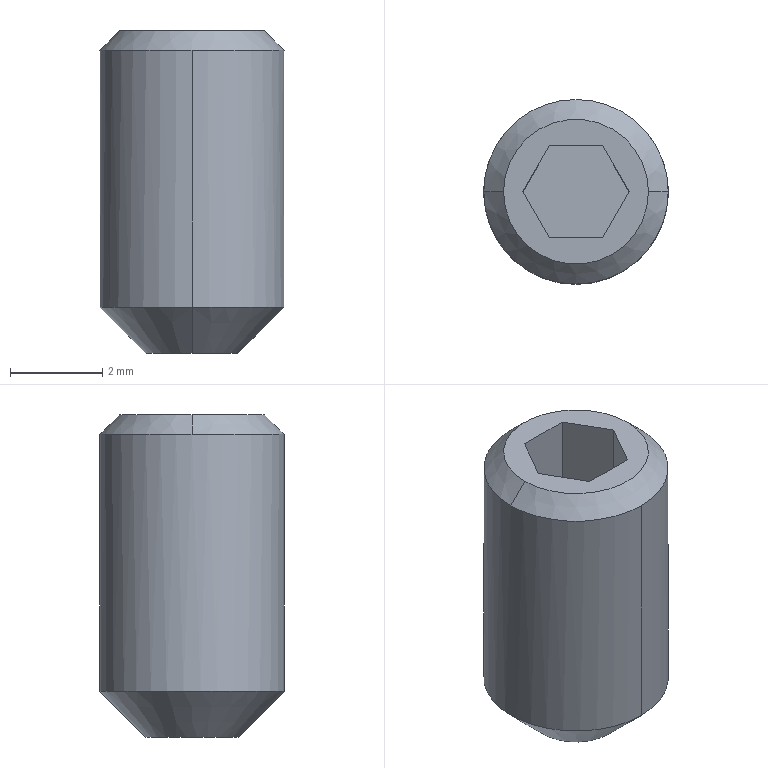Part | SolidWorks | features BaseBody 1 | 1 solid | 16 faces | box 4 x 4 x 7 mm | volume 66.624 mm3 | plane 8 | cone 6 | cylinder 2 | commonest cylinder face diameters 4 x2
STEP:
#1=CARTESIAN_POINT('',(26.15,63.,64.471));
#2=VERTEX_POINT('',#1);
#3=CARTESIAN_POINT('',(24.15,61.,64.471));
#4=VERTEX_POINT('',#3);
#5=CARTESIAN_POINT('',(24.15,63.,64.471));
#6=DIRECTION('',(0.,0.,-1.));
#7=DIRECTION('',(0.,1.,0.));
#8=AXIS2_PLACEMENT_3D('',#5,#6,#7);
#9=CIRCLE('',#8,2.);
#10=EDGE_CURVE('',#2,#4,#9,.T.);
#11=ORIENTED_EDGE('',*,*,#10,.T.);
#12=CARTESIAN_POINT('',(24.15,61.,58.9));
#13=VERTEX_POINT('',#12);
#14=CARTESIAN_POINT('',(24.15,61.,61.685));
#15=DIRECTION('',(0.,0.,-1.));
#16=VECTOR('',#15,1000.);
#17=LINE('',#14,#16);
#18=EDGE_CURVE('',#4,#13,#17,.T.);
#19=ORIENTED_EDGE('',*,*,#18,.T.);
#20=CARTESIAN_POINT('',(24.15,65.,58.9));
#21=VERTEX_POINT('',#20);
#22=CARTESIAN_POINT('',(24.15,63.,58.9));
#23=DIRECTION('',(0.,0.,1.));
#24=DIRECTION('',(0.,1.,0.));
#25=AXIS2_PLACEMENT_3D('',#22,#23,#24);
#26=CIRCLE('',#25,2.);
#27=EDGE_CURVE('',#13,#21,#26,.T.);
#28=ORIENTED_EDGE('',*,*,#27,.T.);
#29=CARTESIAN_POINT('',(24.15,65.,64.471));
#30=VERTEX_POINT('',#29);
#31=CARTESIAN_POINT('',(24.15,65.,61.685));
#32=DIRECTION('',(0.,0.,-1.));
#33=VECTOR('',#32,1000.);
#34=LINE('',#31,#33);
#35=EDGE_CURVE('',#30,#21,#34,.T.);
#36=ORIENTED_EDGE('',*,*,#35,.F.);
#37=CARTESIAN_POINT('',(24.15,63.,64.471));
#38=DIRECTION('',(0.,0.,-1.));
#39=DIRECTION('',(0.,1.,0.));
#40=AXIS2_PLACEMENT_3D('',#37,#38,#39);
#41=CIRCLE('',#40,2.);
#42=EDGE_CURVE('',#30,#2,#41,.T.);
#43=ORIENTED_EDGE('',*,*,#42,.T.);
#44=EDGE_LOOP('',(#11,#19,#28,#36,#43));
#45=FACE_OUTER_BOUND('',#44,.T.);
#46=CARTESIAN_POINT('',(24.15,63.,61.685));
#47=DIRECTION('',(0.,0.,-1.));
#48=DIRECTION('',(0.,1.,0.));
#49=AXIS2_PLACEMENT_3D('',#46,#47,#48);
#50=CYLINDRICAL_SURFACE('',#49,2.);
#51=ADVANCED_FACE('',(#45),#50,.T.);
#52=CARTESIAN_POINT('',(24.15,62.,57.9));
#53=VERTEX_POINT('',#52);
#54=CARTESIAN_POINT('',(24.15,64.,57.9));
#55=VERTEX_POINT('',#54);
#56=CARTESIAN_POINT('',(24.15,63.,57.9));
#57=DIRECTION('',(0.,0.,1.));
#58=DIRECTION('',(1.,0.,0.));
#59=AXIS2_PLACEMENT_3D('',#56,#57,#58);
#60=CIRCLE('',#59,1.);
#61=EDGE_CURVE('',#53,#55,#60,.T.);
#62=ORIENTED_EDGE('',*,*,#61,.T.);
#63=CARTESIAN_POINT('',(24.15,65.,58.9));
#64=DIRECTION('',(0.,0.7071,0.7071));
#65=VECTOR('',#64,1000.);
#66=LINE('',#63,#65);
#67=EDGE_CURVE('',#55,#21,#66,.T.);
#68=ORIENTED_EDGE('',*,*,#67,.T.);
#69=ORIENTED_EDGE('',*,*,#27,.F.);
#70=CARTESIAN_POINT('',(24.15,61.,58.9));
#71=DIRECTION('',(0.,-0.7071,0.7071));
#72=VECTOR('',#71,1000.);
#73=LINE('',#70,#72);
#74=EDGE_CURVE('',#53,#13,#73,.T.);
#75=ORIENTED_EDGE('',*,*,#74,.F.);
#76=EDGE_LOOP('',(#62,#68,#69,#75));
#77=FACE_OUTER_BOUND('',#76,.T.);
#78=CARTESIAN_POINT('',(24.15,63.,58.9));
#79=DIRECTION('',(0.,0.,1.));
#80=DIRECTION('',(0.,-1.,0.));
#81=AXIS2_PLACEMENT_3D('',#78,#79,#80);
#82=CONICAL_SURFACE('',#81,2.,0.7854);
#83=ADVANCED_FACE('',(#77),#82,.T.);
#84=CARTESIAN_POINT('',(22.579,63.,64.9));
#85=VERTEX_POINT('',#84);
#86=CARTESIAN_POINT('',(25.721,63.,64.9));
#87=VERTEX_POINT('',#86);
#88=CARTESIAN_POINT('',(24.15,63.,64.9));
#89=DIRECTION('',(0.,0.,-1.));
#90=DIRECTION('',(-1.,0.,0.));
#91=AXIS2_PLACEMENT_3D('',#88,#89,#90);
#92=CIRCLE('',#91,1.571);
#93=EDGE_CURVE('',#85,#87,#92,.T.);
#94=ORIENTED_EDGE('',*,*,#93,.T.);
#95=CARTESIAN_POINT('',(26.15,63.,64.471));
#96=DIRECTION('',(0.7071,0.,-0.7071));
#97=VECTOR('',#96,1000.);
#98=LINE('',#95,#97);
#99=EDGE_CURVE('',#87,#2,#98,.T.);
#100=ORIENTED_EDGE('',*,*,#99,.T.);
#101=ORIENTED_EDGE('',*,*,#42,.F.);
#102=CARTESIAN_POINT('',(22.15,63.,64.471));
#103=VERTEX_POINT('',#102);
#104=CARTESIAN_POINT('',(24.15,63.,64.471));
#105=DIRECTION('',(0.,0.,-1.));
#106=DIRECTION('',(0.,1.,0.));
#107=AXIS2_PLACEMENT_3D('',#104,#105,#106);
#108=CIRCLE('',#107,2.);
#109=EDGE_CURVE('',#103,#30,#108,.T.);
#110=ORIENTED_EDGE('',*,*,#109,.F.);
#111=CARTESIAN_POINT('',(22.15,63.,64.471));
#112=DIRECTION('',(-0.7071,0.,-0.7071));
#113=VECTOR('',#112,1000.);
#114=LINE('',#111,#113);
#115=EDGE_CURVE('',#85,#103,#114,.T.);
#116=ORIENTED_EDGE('',*,*,#115,.F.);
#117=EDGE_LOOP('',(#94,#100,#101,#110,#116));
#118=FACE_OUTER_BOUND('',#117,.T.);
#119=CARTESIAN_POINT('',(24.15,63.,64.471));
#120=DIRECTION('',(0.,0.,-1.));
#121=DIRECTION('',(-1.,0.,0.));
#122=AXIS2_PLACEMENT_3D('',#119,#120,#121);
#123=CONICAL_SURFACE('',#122,2.,0.7854);
#124=ADVANCED_FACE('',(#118),#123,.T.);
#125=CARTESIAN_POINT('',(24.15,63.,58.477));
#126=VERTEX_POINT('',#125);
#127=CARTESIAN_POINT('',(24.15,64.,57.9));
#128=DIRECTION('',(0.,0.866,-0.5));
#129=VECTOR('',#128,1000.);
#130=LINE('',#127,#129);
#131=EDGE_CURVE('',#126,#55,#130,.T.);
#132=ORIENTED_EDGE('',*,*,#131,.F.);
#133=CARTESIAN_POINT('',(24.15,62.,57.9));
#134=DIRECTION('',(0.,-0.866,-0.5));
#135=VECTOR('',#134,1000.);
#136=LINE('',#133,#135);
#137=EDGE_CURVE('',#126,#53,#136,.T.);
#138=ORIENTED_EDGE('',*,*,#137,.T.);
#139=CARTESIAN_POINT('',(24.15,63.,57.9));
#140=DIRECTION('',(0.,0.,1.));
#141=DIRECTION('',(1.,0.,0.));
#142=AXIS2_PLACEMENT_3D('',#139,#140,#141);
#143=CIRCLE('',#142,1.);
#144=EDGE_CURVE('',#55,#53,#143,.T.);
#145=ORIENTED_EDGE('',*,*,#144,.F.);
#146=EDGE_LOOP('',(#132,#138,#145));
#147=FACE_OUTER_BOUND('',#146,.T.);
#148=CARTESIAN_POINT('',(24.15,63.,57.9));
#149=DIRECTION('',(0.,0.,-1.));
#150=DIRECTION('',(0.,1.,0.));
#151=AXIS2_PLACEMENT_3D('',#148,#149,#150);
#152=CONICAL_SURFACE('',#151,1.,1.047);
#153=ADVANCED_FACE('',(#147),#152,.F.);
#154=ORIENTED_EDGE('',*,*,#18,.F.);
#155=CARTESIAN_POINT('',(24.15,63.,64.471));
#156=DIRECTION('',(0.,0.,-1.));
#157=DIRECTION('',(0.,1.,0.));
#158=AXIS2_PLACEMENT_3D('',#155,#156,#157);
#159=CIRCLE('',#158,2.);
#160=EDGE_CURVE('',#4,#103,#159,.T.);
#161=ORIENTED_EDGE('',*,*,#160,.T.);
#162=ORIENTED_EDGE('',*,*,#109,.T.);
#163=ORIENTED_EDGE('',*,*,#35,.T.);
#164=CARTESIAN_POINT('',(24.15,63.,58.9));
#165=DIRECTION('',(0.,0.,1.));
#166=DIRECTION('',(0.,1.,0.));
#167=AXIS2_PLACEMENT_3D('',#164,#165,#166);
#168=CIRCLE('',#167,2.);
#169=EDGE_CURVE('',#21,#13,#168,.T.);
#170=ORIENTED_EDGE('',*,*,#169,.T.);
#171=EDGE_LOOP('',(#154,#161,#162,#163,#170));
#172=FACE_OUTER_BOUND('',#171,.T.);
#173=CARTESIAN_POINT('',(24.15,63.,61.685));
#174=DIRECTION('',(0.,0.,-1.));
#175=DIRECTION('',(0.,1.,0.));
#176=AXIS2_PLACEMENT_3D('',#173,#174,#175);
#177=CYLINDRICAL_SURFACE('',#176,2.);
#178=ADVANCED_FACE('',(#172),#177,.T.);
#179=ORIENTED_EDGE('',*,*,#67,.F.);
#180=ORIENTED_EDGE('',*,*,#144,.T.);
#181=ORIENTED_EDGE('',*,*,#74,.T.);
#182=ORIENTED_EDGE('',*,*,#169,.F.);
#183=EDGE_LOOP('',(#179,#180,#181,#182));
#184=FACE_OUTER_BOUND('',#183,.T.);
#185=CARTESIAN_POINT('',(24.15,63.,58.9));
#186=DIRECTION('',(0.,0.,1.));
#187=DIRECTION('',(0.,-1.,0.));
#188=AXIS2_PLACEMENT_3D('',#185,#186,#187);
#189=CONICAL_SURFACE('',#188,2.,0.7854);
#190=ADVANCED_FACE('',(#184),#189,.T.);
#191=ORIENTED_EDGE('',*,*,#99,.F.);
#192=CARTESIAN_POINT('',(24.15,63.,64.9));
#193=DIRECTION('',(0.,0.,-1.));
#194=DIRECTION('',(-1.,0.,0.));
#195=AXIS2_PLACEMENT_3D('',#192,#193,#194);
#196=CIRCLE('',#195,1.571);
#197=EDGE_CURVE('',#87,#85,#196,.T.);
#198=ORIENTED_EDGE('',*,*,#197,.T.);
#199=ORIENTED_EDGE('',*,*,#115,.T.);
#200=ORIENTED_EDGE('',*,*,#160,.F.);
#201=ORIENTED_EDGE('',*,*,#10,.F.);
#202=EDGE_LOOP('',(#191,#198,#199,#200,#201));
#203=FACE_OUTER_BOUND('',#202,.T.);
#204=CARTESIAN_POINT('',(24.15,63.,64.471));
#205=DIRECTION('',(0.,0.,-1.));
#206=DIRECTION('',(-1.,0.,0.));
#207=AXIS2_PLACEMENT_3D('',#204,#205,#206);
#208=CONICAL_SURFACE('',#207,2.,0.7854);
#209=ADVANCED_FACE('',(#203),#208,.T.);
#210=ORIENTED_EDGE('',*,*,#137,.F.);
#211=ORIENTED_EDGE('',*,*,#131,.T.);
#212=ORIENTED_EDGE('',*,*,#61,.F.);
#213=EDGE_LOOP('',(#210,#211,#212));
#214=FACE_OUTER_BOUND('',#213,.T.);
#215=CARTESIAN_POINT('',(24.15,63.,57.9));
#216=DIRECTION('',(0.,0.,-1.));
#217=DIRECTION('',(0.,1.,0.));
#218=AXIS2_PLACEMENT_3D('',#215,#216,#217);
#219=CONICAL_SURFACE('',#218,1.,1.047);
#220=ADVANCED_FACE('',(#214),#219,.F.);
#221=ORIENTED_EDGE('',*,*,#93,.F.);
#222=ORIENTED_EDGE('',*,*,#197,.F.);
#223=EDGE_LOOP('',(#221,#222));
#224=FACE_OUTER_BOUND('',#223,.T.);
#225=CARTESIAN_POINT('',(24.727,62.,64.9));
#226=VERTEX_POINT('',#225);
#227=CARTESIAN_POINT('',(25.305,63.,64.9));
#228=VERTEX_POINT('',#227);
#229=CARTESIAN_POINT('',(25.016,62.5,64.9));
#230=DIRECTION('',(0.5,0.866,0.));
#231=VECTOR('',#230,1000.);
#232=LINE('',#229,#231);
#233=EDGE_CURVE('',#226,#228,#232,.T.);
#234=ORIENTED_EDGE('',*,*,#233,.F.);
#235=CARTESIAN_POINT('',(23.573,62.,64.9));
#236=VERTEX_POINT('',#235);
#237=CARTESIAN_POINT('',(24.15,62.,64.9));
#238=DIRECTION('',(1.,0.,0.));
#239=VECTOR('',#238,1000.);
#240=LINE('',#237,#239);
#241=EDGE_CURVE('',#236,#226,#240,.T.);
#242=ORIENTED_EDGE('',*,*,#241,.F.);
#243=CARTESIAN_POINT('',(22.995,63.,64.9));
#244=VERTEX_POINT('',#243);
#245=CARTESIAN_POINT('',(23.284,62.5,64.9));
#246=DIRECTION('',(0.5,-0.866,0.));
#247=VECTOR('',#246,1000.);
#248=LINE('',#245,#247);
#249=EDGE_CURVE('',#244,#236,#248,.T.);
#250=ORIENTED_EDGE('',*,*,#249,.F.);
#251=CARTESIAN_POINT('',(23.573,64.,64.9));
#252=VERTEX_POINT('',#251);
#253=CARTESIAN_POINT('',(23.284,63.5,64.9));
#254=DIRECTION('',(-0.5,-0.866,0.));
#255=VECTOR('',#254,1000.);
#256=LINE('',#253,#255);
#257=EDGE_CURVE('',#252,#244,#256,.T.);
#258=ORIENTED_EDGE('',*,*,#257,.F.);
#259=CARTESIAN_POINT('',(24.727,64.,64.9));
#260=VERTEX_POINT('',#259);
#261=CARTESIAN_POINT('',(24.15,64.,64.9));
#262=DIRECTION('',(-1.,0.,0.));
#263=VECTOR('',#262,1000.);
#264=LINE('',#261,#263);
#265=EDGE_CURVE('',#260,#252,#264,.T.);
#266=ORIENTED_EDGE('',*,*,#265,.F.);
#267=CARTESIAN_POINT('',(25.305,63.,64.9));
#268=DIRECTION('',(-0.5,0.866,0.));
#269=VECTOR('',#268,1000.);
#270=LINE('',#267,#269);
#271=EDGE_CURVE('',#228,#260,#270,.T.);
#272=ORIENTED_EDGE('',*,*,#271,.F.);
#273=EDGE_LOOP('',(#234,#242,#250,#258,#266,#272));
#274=FACE_BOUND('',#273,.T.);
#275=CARTESIAN_POINT('',(24.15,63.,64.9));
#276=DIRECTION('',(0.,0.,-1.));
#277=DIRECTION('',(0.,1.,0.));
#278=AXIS2_PLACEMENT_3D('',#275,#276,#277);
#279=PLANE('',#278);
#280=ADVANCED_FACE('',(#224,#274),#279,.F.);
#281=CARTESIAN_POINT('',(25.305,63.,60.736));
#282=VERTEX_POINT('',#281);
#283=CARTESIAN_POINT('',(25.305,63.,62.818));
#284=DIRECTION('',(0.,0.,1.));
#285=VECTOR('',#284,1000.);
#286=LINE('',#283,#285);
#287=EDGE_CURVE('',#282,#228,#286,.T.);
#288=ORIENTED_EDGE('',*,*,#287,.T.);
#289=ORIENTED_EDGE('',*,*,#271,.T.);
#290=CARTESIAN_POINT('',(24.727,64.,60.736));
#291=VERTEX_POINT('',#290);
#292=CARTESIAN_POINT('',(24.727,64.,62.818));
#293=DIRECTION('',(0.,0.,-1.));
#294=VECTOR('',#293,1000.);
#295=LINE('',#292,#294);
#296=EDGE_CURVE('',#260,#291,#295,.T.);
#297=ORIENTED_EDGE('',*,*,#296,.T.);
#298=CARTESIAN_POINT('',(25.016,63.5,60.736));
#299=DIRECTION('',(0.5,-0.866,0.));
#300=VECTOR('',#299,1000.);
#301=LINE('',#298,#300);
#302=EDGE_CURVE('',#291,#282,#301,.T.);
#303=ORIENTED_EDGE('',*,*,#302,.T.);
#304=EDGE_LOOP('',(#288,#289,#297,#303));
#305=FACE_OUTER_BOUND('',#304,.T.);
#306=CARTESIAN_POINT('',(25.016,63.5,62.818));
#307=DIRECTION('',(-0.866,-0.5,0.));
#308=DIRECTION('',(0.5,-0.866,0.));
#309=AXIS2_PLACEMENT_3D('',#306,#307,#308);
#310=PLANE('',#309);
#311=ADVANCED_FACE('',(#305),#310,.T.);
#312=CARTESIAN_POINT('',(24.727,62.,60.736));
#313=VERTEX_POINT('',#312);
#314=CARTESIAN_POINT('',(24.727,62.,62.818));
#315=DIRECTION('',(0.,0.,1.));
#316=VECTOR('',#315,1000.);
#317=LINE('',#314,#316);
#318=EDGE_CURVE('',#313,#226,#317,.T.);
#319=ORIENTED_EDGE('',*,*,#318,.T.);
#320=ORIENTED_EDGE('',*,*,#233,.T.);
#321=ORIENTED_EDGE('',*,*,#287,.F.);
#322=CARTESIAN_POINT('',(25.016,62.5,60.736));
#323=DIRECTION('',(-0.5,-0.866,0.));
#324=VECTOR('',#323,1000.);
#325=LINE('',#322,#324);
#326=EDGE_CURVE('',#282,#313,#325,.T.);
#327=ORIENTED_EDGE('',*,*,#326,.T.);
#328=EDGE_LOOP('',(#319,#320,#321,#327));
#329=FACE_OUTER_BOUND('',#328,.T.);
#330=CARTESIAN_POINT('',(25.016,62.5,62.818));
#331=DIRECTION('',(-0.866,0.5,0.));
#332=DIRECTION('',(-0.5,-0.866,0.));
#333=AXIS2_PLACEMENT_3D('',#330,#331,#332);
#334=PLANE('',#333);
#335=ADVANCED_FACE('',(#329),#334,.T.);
#336=ORIENTED_EDGE('',*,*,#326,.F.);
#337=ORIENTED_EDGE('',*,*,#302,.F.);
#338=CARTESIAN_POINT('',(23.573,64.,60.736));
#339=VERTEX_POINT('',#338);
#340=CARTESIAN_POINT('',(24.15,64.,60.736));
#341=DIRECTION('',(1.,0.,0.));
#342=VECTOR('',#341,1000.);
#343=LINE('',#340,#342);
#344=EDGE_CURVE('',#339,#291,#343,.T.);
#345=ORIENTED_EDGE('',*,*,#344,.F.);
#346=CARTESIAN_POINT('',(22.995,63.,60.736));
#347=VERTEX_POINT('',#346);
#348=CARTESIAN_POINT('',(23.284,63.5,60.736));
#349=DIRECTION('',(0.5,0.866,0.));
#350=VECTOR('',#349,1000.);
#351=LINE('',#348,#350);
#352=EDGE_CURVE('',#347,#339,#351,.T.);
#353=ORIENTED_EDGE('',*,*,#352,.F.);
#354=CARTESIAN_POINT('',(23.573,62.,60.736));
#355=VERTEX_POINT('',#354);
#356=CARTESIAN_POINT('',(23.284,62.5,60.736));
#357=DIRECTION('',(-0.5,0.866,0.));
#358=VECTOR('',#357,1000.);
#359=LINE('',#356,#358);
#360=EDGE_CURVE('',#355,#347,#359,.T.);
#361=ORIENTED_EDGE('',*,*,#360,.F.);
#362=CARTESIAN_POINT('',(24.15,62.,60.736));
#363=DIRECTION('',(-1.,0.,0.));
#364=VECTOR('',#363,1000.);
#365=LINE('',#362,#364);
#366=EDGE_CURVE('',#313,#355,#365,.T.);
#367=ORIENTED_EDGE('',*,*,#366,.F.);
#368=EDGE_LOOP('',(#336,#337,#345,#353,#361,#367));
#369=FACE_OUTER_BOUND('',#368,.T.);
#370=CARTESIAN_POINT('',(24.15,63.,60.736));
#371=DIRECTION('',(0.,0.,-1.));
#372=DIRECTION('',(0.,1.,0.));
#373=AXIS2_PLACEMENT_3D('',#370,#371,#372);
#374=PLANE('',#373);
#375=ADVANCED_FACE('',(#369),#374,.F.);
#376=ORIENTED_EDGE('',*,*,#296,.F.);
#377=ORIENTED_EDGE('',*,*,#265,.T.);
#378=CARTESIAN_POINT('',(23.573,64.,62.818));
#379=DIRECTION('',(0.,0.,-1.));
#380=VECTOR('',#379,1000.);
#381=LINE('',#378,#380);
#382=EDGE_CURVE('',#252,#339,#381,.T.);
#383=ORIENTED_EDGE('',*,*,#382,.T.);
#384=ORIENTED_EDGE('',*,*,#344,.T.);
#385=EDGE_LOOP('',(#376,#377,#383,#384));
#386=FACE_OUTER_BOUND('',#385,.T.);
#387=CARTESIAN_POINT('',(24.15,64.,62.818));
#388=DIRECTION('',(0.,-1.,0.));
#389=DIRECTION('',(0.,0.,-1.));
#390=AXIS2_PLACEMENT_3D('',#387,#388,#389);
#391=PLANE('',#390);
#392=ADVANCED_FACE('',(#386),#391,.T.);
#393=CARTESIAN_POINT('',(23.573,62.,62.818));
#394=DIRECTION('',(0.,0.,1.));
#395=VECTOR('',#394,1000.);
#396=LINE('',#393,#395);
#397=EDGE_CURVE('',#355,#236,#396,.T.);
#398=ORIENTED_EDGE('',*,*,#397,.T.);
#399=ORIENTED_EDGE('',*,*,#241,.T.);
#400=ORIENTED_EDGE('',*,*,#318,.F.);
#401=ORIENTED_EDGE('',*,*,#366,.T.);
#402=EDGE_LOOP('',(#398,#399,#400,#401));
#403=FACE_OUTER_BOUND('',#402,.T.);
#404=CARTESIAN_POINT('',(24.15,62.,62.818));
#405=DIRECTION('',(0.,1.,0.));
#406=DIRECTION('',(0.,0.,1.));
#407=AXIS2_PLACEMENT_3D('',#404,#405,#406);
#408=PLANE('',#407);
#409=ADVANCED_FACE('',(#403),#408,.T.);
#410=ORIENTED_EDGE('',*,*,#382,.F.);
#411=ORIENTED_EDGE('',*,*,#257,.T.);
#412=CARTESIAN_POINT('',(22.995,63.,62.818));
#413=DIRECTION('',(0.,0.,-1.));
#414=VECTOR('',#413,1000.);
#415=LINE('',#412,#414);
#416=EDGE_CURVE('',#244,#347,#415,.T.);
#417=ORIENTED_EDGE('',*,*,#416,.T.);
#418=ORIENTED_EDGE('',*,*,#352,.T.);
#419=EDGE_LOOP('',(#410,#411,#417,#418));
#420=FACE_OUTER_BOUND('',#419,.T.);
#421=CARTESIAN_POINT('',(23.284,63.5,62.818));
#422=DIRECTION('',(0.866,-0.5,0.));
#423=DIRECTION('',(0.5,0.866,0.));
#424=AXIS2_PLACEMENT_3D('',#421,#422,#423);
#425=PLANE('',#424);
#426=ADVANCED_FACE('',(#420),#425,.T.);
#427=ORIENTED_EDGE('',*,*,#416,.F.);
#428=ORIENTED_EDGE('',*,*,#249,.T.);
#429=ORIENTED_EDGE('',*,*,#397,.F.);
#430=ORIENTED_EDGE('',*,*,#360,.T.);
#431=EDGE_LOOP('',(#427,#428,#429,#430));
#432=FACE_OUTER_BOUND('',#431,.T.);
#433=CARTESIAN_POINT('',(23.284,62.5,62.818));
#434=DIRECTION('',(0.866,0.5,0.));
#435=DIRECTION('',(-0.5,0.866,0.));
#436=AXIS2_PLACEMENT_3D('',#433,#434,#435);
#437=PLANE('',#436);
#438=ADVANCED_FACE('',(#432),#437,.T.);
#439=CLOSED_SHELL('',(#51,#83,#124,#153,#178,#190,#209,#220,#280,#311,#335,#375,#392,#409,#426,#438));
#440=MANIFOLD_SOLID_BREP('',#439);
#441=CARTESIAN_POINT('',(0.,0.,0.));
#442=DIRECTION('',(0.,0.,1.));
#443=DIRECTION('',(1.,0.,0.));
#444=AXIS2_PLACEMENT_3D('',#441,#442,#443);
#445=(LENGTH_UNIT()NAMED_UNIT(*)SI_UNIT(.MILLI.,.METRE.));
#446=UNCERTAINTY_MEASURE_WITH_UNIT(LENGTH_MEASURE(0.00001),#445,'','');
#447=(NAMED_UNIT(*)PLANE_ANGLE_UNIT()SI_UNIT($,.RADIAN.));
#448=(NAMED_UNIT(*)SI_UNIT($,.STERADIAN.)SOLID_ANGLE_UNIT());
#449=(GEOMETRIC_REPRESENTATION_CONTEXT(3)GLOBAL_UNCERTAINTY_ASSIGNED_CONTEXT((#446))GLOBAL_UNIT_ASSIGNED_CONTEXT((#445,#447,#448))REPRESENTATION_CONTEXT('',''));
#450=ADVANCED_BREP_SHAPE_REPRESENTATION('',(#440,#444),#449);